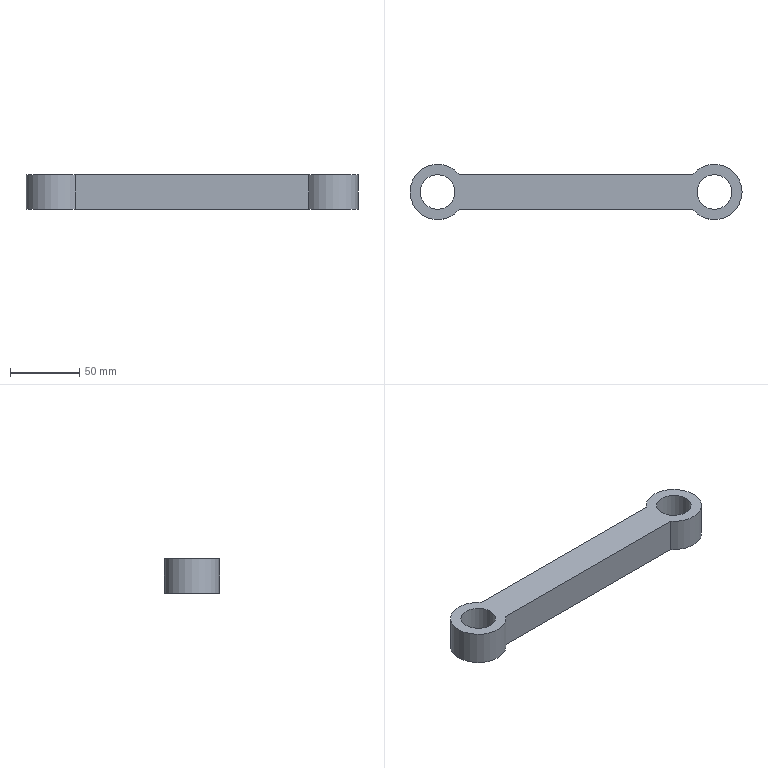Part | NX | features DATUM_CSYS 2, SIMPLE HOLE 2, EXTRUDE 1, HOLE PACKAGE 1, SKETCH 1 | 1 solid | 8 faces | box 240 x 40 x 25 mm | volume 140028 mm3 | cylinder 4 | plane 4 | commonest cylinder face diameters 25 x2 40 x2
STEP:
#1=CARTESIAN_POINT('',(15.612,12.5,-12.5));
#2=VERTEX_POINT('',#1);
#3=CARTESIAN_POINT('',(15.612,-12.5,-12.5));
#4=VERTEX_POINT('',#3);
#5=CARTESIAN_POINT('',(0.,0.,-12.5));
#6=DIRECTION('',(0.,0.,1.));
#7=DIRECTION('',(1.,0.,0.));
#8=AXIS2_PLACEMENT_3D('',#5,#6,#7);
#9=CIRCLE('',#8,20.);
#10=EDGE_CURVE('',#2,#4,#9,.T.);
#11=ORIENTED_EDGE('',*,*,#10,.T.);
#12=CARTESIAN_POINT('',(15.612,-12.5,12.5));
#13=VERTEX_POINT('',#12);
#14=CARTESIAN_POINT('',(15.612,-12.5,12.5));
#15=DIRECTION('',(0.,0.,-1.));
#16=VECTOR('',#15,1000.);
#17=LINE('',#14,#16);
#18=EDGE_CURVE('',#13,#4,#17,.T.);
#19=ORIENTED_EDGE('',*,*,#18,.F.);
#20=CARTESIAN_POINT('',(15.612,12.5,12.5));
#21=VERTEX_POINT('',#20);
#22=CARTESIAN_POINT('',(0.,0.,12.5));
#23=DIRECTION('',(0.,0.,1.));
#24=DIRECTION('',(1.,0.,0.));
#25=AXIS2_PLACEMENT_3D('',#22,#23,#24);
#26=CIRCLE('',#25,20.);
#27=EDGE_CURVE('',#21,#13,#26,.T.);
#28=ORIENTED_EDGE('',*,*,#27,.F.);
#29=CARTESIAN_POINT('',(15.612,12.5,12.5));
#30=DIRECTION('',(0.,0.,-1.));
#31=VECTOR('',#30,1000.);
#32=LINE('',#29,#31);
#33=EDGE_CURVE('',#21,#2,#32,.T.);
#34=ORIENTED_EDGE('',*,*,#33,.T.);
#35=EDGE_LOOP('',(#11,#19,#28,#34));
#36=FACE_BOUND('',#35,.T.);
#37=CARTESIAN_POINT('',(0.,0.,12.5));
#38=DIRECTION('',(0.,0.,-1.));
#39=DIRECTION('',(-1.,0.,0.));
#40=AXIS2_PLACEMENT_3D('',#37,#38,#39);
#41=CYLINDRICAL_SURFACE('',#40,20.);
#42=ADVANCED_FACE('',(#36),#41,.T.);
#43=CARTESIAN_POINT('',(184.388,-12.5,-12.5));
#44=VERTEX_POINT('',#43);
#45=CARTESIAN_POINT('',(15.612,-12.5,-12.5));
#46=DIRECTION('',(1.,0.,0.));
#47=VECTOR('',#46,1000.);
#48=LINE('',#45,#47);
#49=EDGE_CURVE('',#4,#44,#48,.T.);
#50=ORIENTED_EDGE('',*,*,#49,.T.);
#51=CARTESIAN_POINT('',(184.388,-12.5,12.5));
#52=VERTEX_POINT('',#51);
#53=CARTESIAN_POINT('',(184.388,-12.5,12.5));
#54=DIRECTION('',(0.,0.,-1.));
#55=VECTOR('',#54,1000.);
#56=LINE('',#53,#55);
#57=EDGE_CURVE('',#52,#44,#56,.T.);
#58=ORIENTED_EDGE('',*,*,#57,.F.);
#59=CARTESIAN_POINT('',(15.612,-12.5,12.5));
#60=DIRECTION('',(1.,0.,0.));
#61=VECTOR('',#60,1000.);
#62=LINE('',#59,#61);
#63=EDGE_CURVE('',#13,#52,#62,.T.);
#64=ORIENTED_EDGE('',*,*,#63,.F.);
#65=ORIENTED_EDGE('',*,*,#18,.T.);
#66=EDGE_LOOP('',(#50,#58,#64,#65));
#67=FACE_BOUND('',#66,.T.);
#68=CARTESIAN_POINT('',(15.612,-12.5,12.5));
#69=DIRECTION('',(0.,1.,0.));
#70=DIRECTION('',(-1.,0.,0.));
#71=AXIS2_PLACEMENT_3D('',#68,#69,#70);
#72=PLANE('',#71);
#73=ADVANCED_FACE('',(#67),#72,.F.);
#74=CARTESIAN_POINT('',(184.388,12.5,-12.5));
#75=VERTEX_POINT('',#74);
#76=CARTESIAN_POINT('',(200.,0.,-12.5));
#77=DIRECTION('',(0.,0.,1.));
#78=DIRECTION('',(-1.,0.,0.));
#79=AXIS2_PLACEMENT_3D('',#76,#77,#78);
#80=CIRCLE('',#79,20.);
#81=EDGE_CURVE('',#44,#75,#80,.T.);
#82=ORIENTED_EDGE('',*,*,#81,.T.);
#83=CARTESIAN_POINT('',(184.388,12.5,12.5));
#84=VERTEX_POINT('',#83);
#85=CARTESIAN_POINT('',(184.388,12.5,12.5));
#86=DIRECTION('',(0.,0.,-1.));
#87=VECTOR('',#86,1000.);
#88=LINE('',#85,#87);
#89=EDGE_CURVE('',#84,#75,#88,.T.);
#90=ORIENTED_EDGE('',*,*,#89,.F.);
#91=CARTESIAN_POINT('',(200.,0.,12.5));
#92=DIRECTION('',(0.,0.,1.));
#93=DIRECTION('',(-1.,0.,0.));
#94=AXIS2_PLACEMENT_3D('',#91,#92,#93);
#95=CIRCLE('',#94,20.);
#96=EDGE_CURVE('',#52,#84,#95,.T.);
#97=ORIENTED_EDGE('',*,*,#96,.F.);
#98=ORIENTED_EDGE('',*,*,#57,.T.);
#99=EDGE_LOOP('',(#82,#90,#97,#98));
#100=FACE_BOUND('',#99,.T.);
#101=CARTESIAN_POINT('',(200.,0.,12.5));
#102=DIRECTION('',(0.,0.,-1.));
#103=DIRECTION('',(-1.,0.,0.));
#104=AXIS2_PLACEMENT_3D('',#101,#102,#103);
#105=CYLINDRICAL_SURFACE('',#104,20.);
#106=ADVANCED_FACE('',(#100),#105,.T.);
#107=CARTESIAN_POINT('',(184.388,12.5,-12.5));
#108=DIRECTION('',(-1.,0.,0.));
#109=VECTOR('',#108,1000.);
#110=LINE('',#107,#109);
#111=EDGE_CURVE('',#75,#2,#110,.T.);
#112=ORIENTED_EDGE('',*,*,#111,.T.);
#113=ORIENTED_EDGE('',*,*,#33,.F.);
#114=CARTESIAN_POINT('',(184.388,12.5,12.5));
#115=DIRECTION('',(-1.,0.,0.));
#116=VECTOR('',#115,1000.);
#117=LINE('',#114,#116);
#118=EDGE_CURVE('',#84,#21,#117,.T.);
#119=ORIENTED_EDGE('',*,*,#118,.F.);
#120=ORIENTED_EDGE('',*,*,#89,.T.);
#121=EDGE_LOOP('',(#112,#113,#119,#120));
#122=FACE_BOUND('',#121,.T.);
#123=CARTESIAN_POINT('',(184.388,12.5,12.5));
#124=DIRECTION('',(0.,-1.,0.));
#125=DIRECTION('',(0.,0.,-1.));
#126=AXIS2_PLACEMENT_3D('',#123,#124,#125);
#127=PLANE('',#126);
#128=ADVANCED_FACE('',(#122),#127,.F.);
#129=CARTESIAN_POINT('',(187.5,0.,12.5));
#130=VERTEX_POINT('',#129);
#131=CARTESIAN_POINT('',(200.,0.,12.5));
#132=DIRECTION('',(0.,0.,-1.));
#133=DIRECTION('',(-1.,0.,0.));
#134=AXIS2_PLACEMENT_3D('',#131,#132,#133);
#135=CIRCLE('',#134,12.5);
#136=EDGE_CURVE('',#130,#130,#135,.T.);
#137=ORIENTED_EDGE('',*,*,#136,.T.);
#138=EDGE_LOOP('',(#137));
#139=FACE_BOUND('',#138,.T.);
#140=CARTESIAN_POINT('',(-12.5,0.,12.5));
#141=VERTEX_POINT('',#140);
#142=CARTESIAN_POINT('',(0.,0.,12.5));
#143=DIRECTION('',(0.,0.,-1.));
#144=DIRECTION('',(-1.,0.,0.));
#145=AXIS2_PLACEMENT_3D('',#142,#143,#144);
#146=CIRCLE('',#145,12.5);
#147=EDGE_CURVE('',#141,#141,#146,.T.);
#148=ORIENTED_EDGE('',*,*,#147,.T.);
#149=EDGE_LOOP('',(#148));
#150=FACE_BOUND('',#149,.T.);
#151=ORIENTED_EDGE('',*,*,#27,.T.);
#152=ORIENTED_EDGE('',*,*,#63,.T.);
#153=ORIENTED_EDGE('',*,*,#96,.T.);
#154=ORIENTED_EDGE('',*,*,#118,.T.);
#155=EDGE_LOOP('',(#151,#152,#153,#154));
#156=FACE_BOUND('',#155,.T.);
#157=CARTESIAN_POINT('',(0.,0.,12.5));
#158=DIRECTION('',(0.,0.,1.));
#159=DIRECTION('',(1.,0.,0.));
#160=AXIS2_PLACEMENT_3D('',#157,#158,#159);
#161=PLANE('',#160);
#162=ADVANCED_FACE('',(#139,#150,#156),#161,.T.);
#163=CARTESIAN_POINT('',(212.5,0.,-12.5));
#164=VERTEX_POINT('',#163);
#165=CARTESIAN_POINT('',(200.,0.,-12.5));
#166=DIRECTION('',(0.,0.,1.));
#167=DIRECTION('',(1.,0.,0.));
#168=AXIS2_PLACEMENT_3D('',#165,#166,#167);
#169=CIRCLE('',#168,12.5);
#170=EDGE_CURVE('',#164,#164,#169,.T.);
#171=ORIENTED_EDGE('',*,*,#170,.T.);
#172=EDGE_LOOP('',(#171));
#173=FACE_BOUND('',#172,.T.);
#174=CARTESIAN_POINT('',(12.5,0.,-12.5));
#175=VERTEX_POINT('',#174);
#176=CARTESIAN_POINT('',(0.,0.,-12.5));
#177=DIRECTION('',(0.,0.,1.));
#178=DIRECTION('',(1.,0.,0.));
#179=AXIS2_PLACEMENT_3D('',#176,#177,#178);
#180=CIRCLE('',#179,12.5);
#181=EDGE_CURVE('',#175,#175,#180,.T.);
#182=ORIENTED_EDGE('',*,*,#181,.T.);
#183=EDGE_LOOP('',(#182));
#184=FACE_BOUND('',#183,.T.);
#185=ORIENTED_EDGE('',*,*,#10,.F.);
#186=ORIENTED_EDGE('',*,*,#111,.F.);
#187=ORIENTED_EDGE('',*,*,#81,.F.);
#188=ORIENTED_EDGE('',*,*,#49,.F.);
#189=EDGE_LOOP('',(#185,#186,#187,#188));
#190=FACE_BOUND('',#189,.T.);
#191=CARTESIAN_POINT('',(0.,0.,-12.5));
#192=DIRECTION('',(0.,0.,1.));
#193=DIRECTION('',(1.,0.,0.));
#194=AXIS2_PLACEMENT_3D('',#191,#192,#193);
#195=PLANE('',#194);
#196=ADVANCED_FACE('',(#173,#184,#190),#195,.F.);
#197=ORIENTED_EDGE('',*,*,#147,.F.);
#198=EDGE_LOOP('',(#197));
#199=FACE_BOUND('',#198,.T.);
#200=ORIENTED_EDGE('',*,*,#181,.F.);
#201=EDGE_LOOP('',(#200));
#202=FACE_BOUND('',#201,.T.);
#203=CARTESIAN_POINT('',(0.,0.,12.5));
#204=DIRECTION('',(0.,0.,-1.));
#205=DIRECTION('',(-1.,0.,0.));
#206=AXIS2_PLACEMENT_3D('',#203,#204,#205);
#207=CYLINDRICAL_SURFACE('',#206,12.5);
#208=ADVANCED_FACE('',(#199,#202),#207,.F.);
#209=ORIENTED_EDGE('',*,*,#136,.F.);
#210=EDGE_LOOP('',(#209));
#211=FACE_BOUND('',#210,.T.);
#212=ORIENTED_EDGE('',*,*,#170,.F.);
#213=EDGE_LOOP('',(#212));
#214=FACE_BOUND('',#213,.T.);
#215=CARTESIAN_POINT('',(200.,0.,12.5));
#216=DIRECTION('',(0.,0.,-1.));
#217=DIRECTION('',(-1.,0.,0.));
#218=AXIS2_PLACEMENT_3D('',#215,#216,#217);
#219=CYLINDRICAL_SURFACE('',#218,12.5);
#220=ADVANCED_FACE('',(#211,#214),#219,.F.);
#221=CLOSED_SHELL('',(#42,#73,#106,#128,#162,#196,#208,#220));
#222=MANIFOLD_SOLID_BREP('',#221);
#223=(LENGTH_UNIT()NAMED_UNIT(*)SI_UNIT(.MILLI.,.METRE.));
#224=UNCERTAINTY_MEASURE_WITH_UNIT(LENGTH_MEASURE(0.00001),#223,'','');
#225=(NAMED_UNIT(*)PLANE_ANGLE_UNIT()SI_UNIT($,.RADIAN.));
#226=(NAMED_UNIT(*)SI_UNIT($,.STERADIAN.)SOLID_ANGLE_UNIT());
#227=(GEOMETRIC_REPRESENTATION_CONTEXT(3)GLOBAL_UNCERTAINTY_ASSIGNED_CONTEXT((#224))GLOBAL_UNIT_ASSIGNED_CONTEXT((#223,#225,#226))REPRESENTATION_CONTEXT('',''));
#228=ADVANCED_BREP_SHAPE_REPRESENTATION('',(#222),#227);